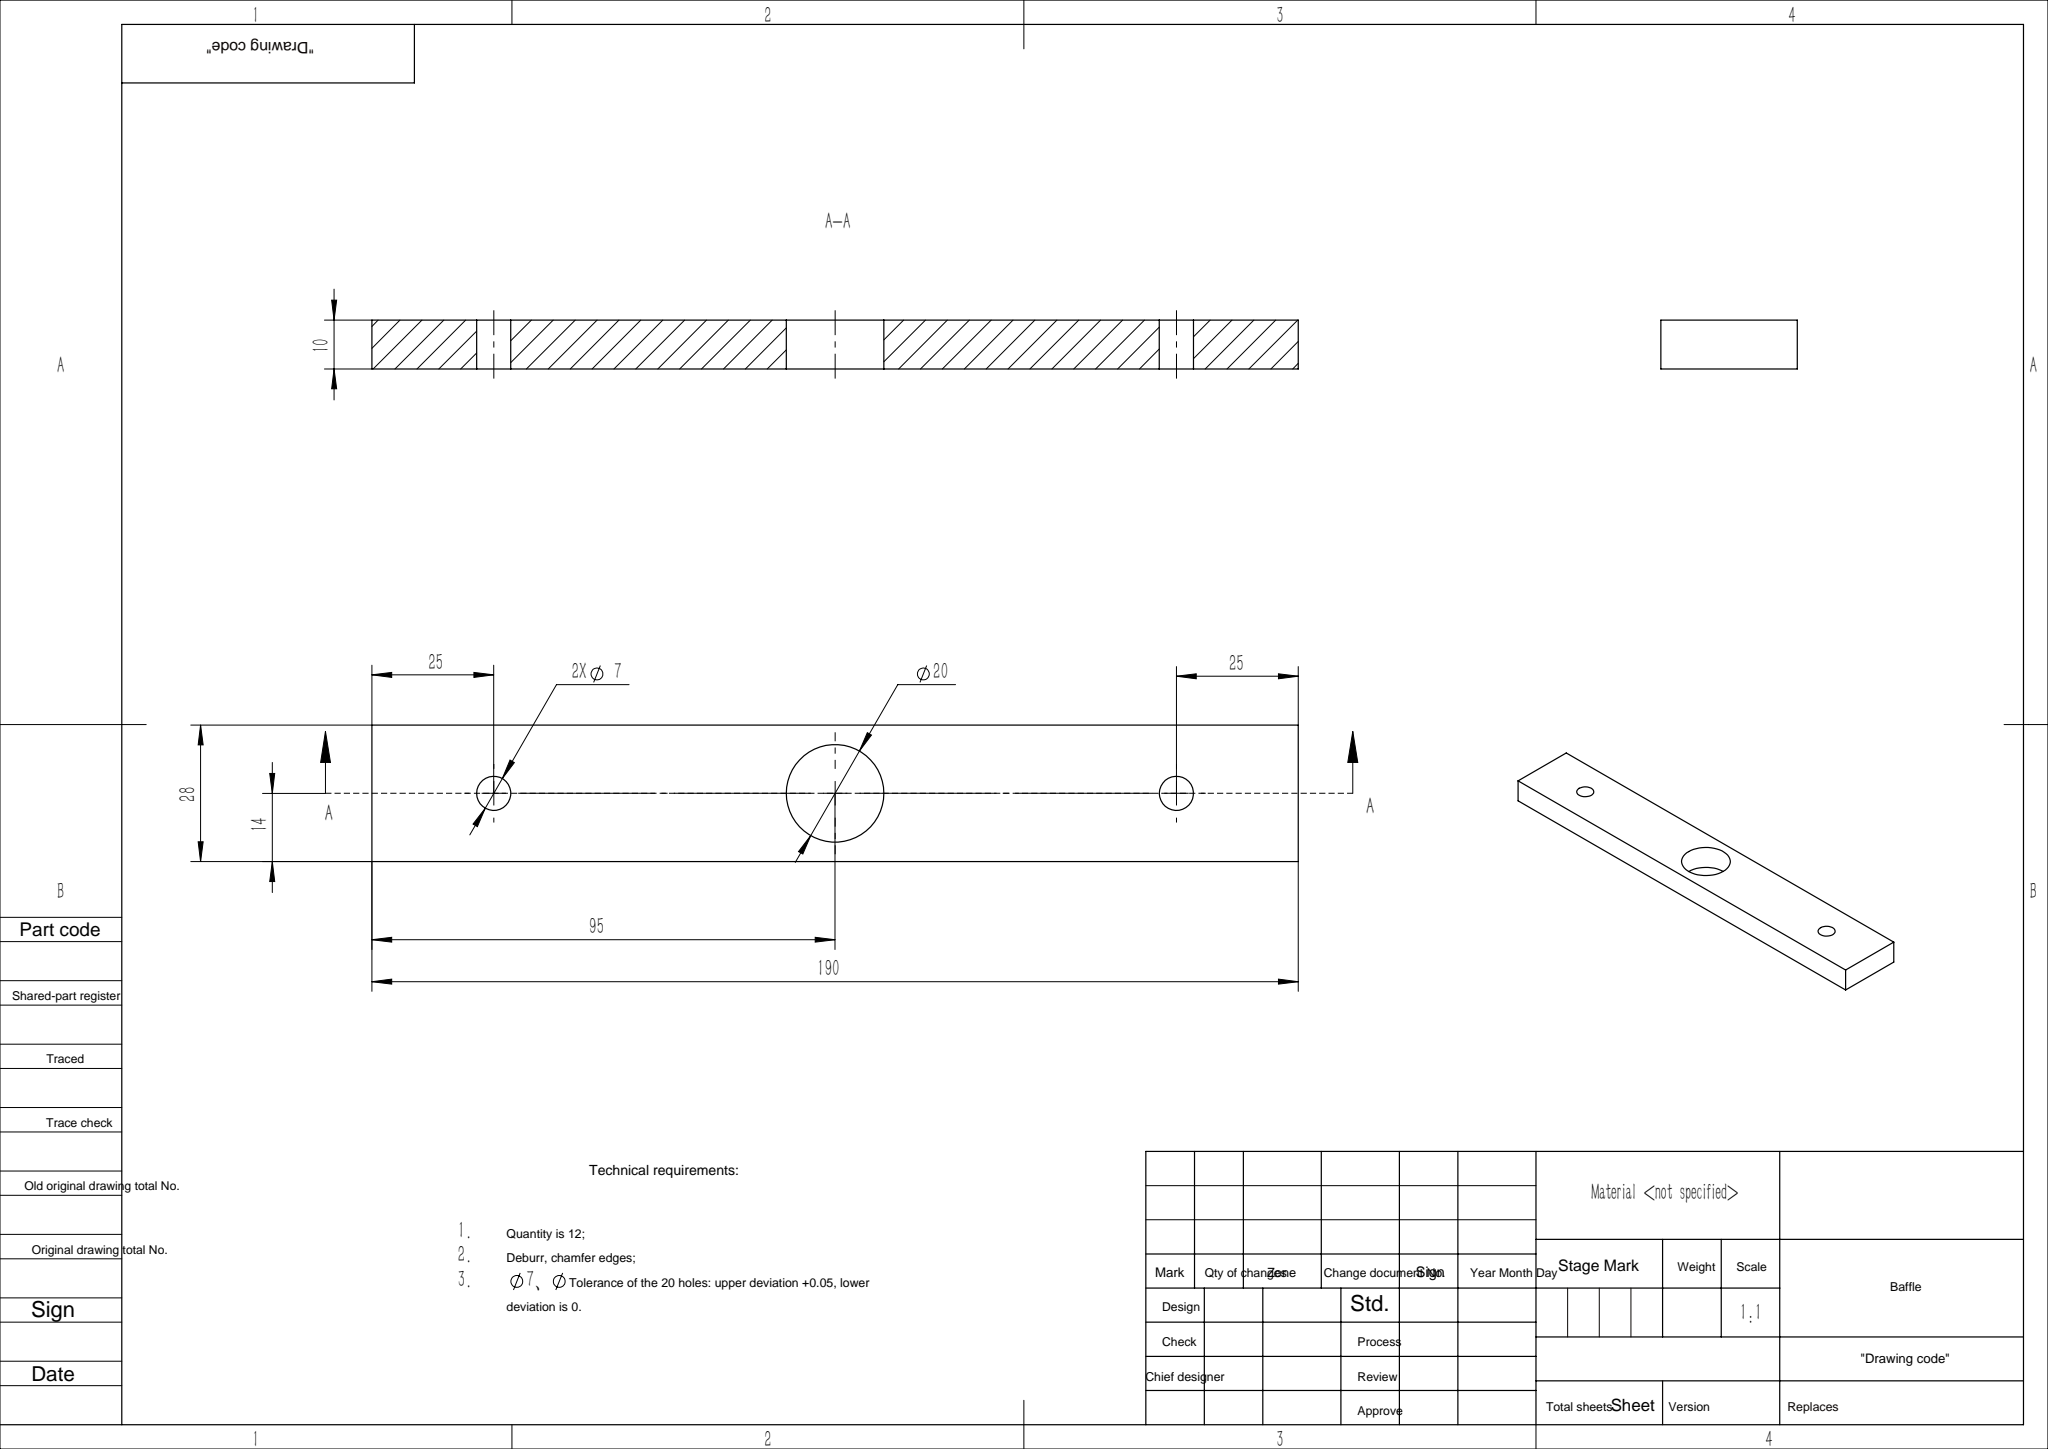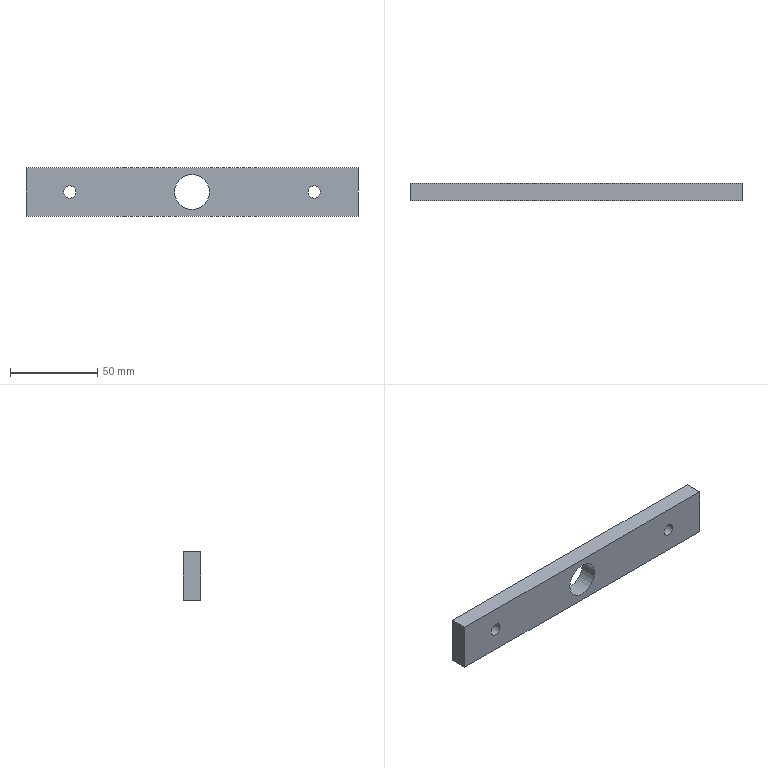Part | SolidWorks | features Cut 1, Extrusion 1 | 1 solid | 12 faces | box 190 x 10 x 28 mm | volume 49289 mm3 | cylinder 6 | plane 6 | commonest cylinder face diameters 7 x4 20 x2
STEP:
#1=CARTESIAN_POINT('',(612.086,1805.,-465.));
#2=VERTEX_POINT('',#1);
#3=CARTESIAN_POINT('',(592.086,1805.,-465.));
#4=VERTEX_POINT('',#3);
#5=CARTESIAN_POINT('',(602.086,1805.,-465.));
#6=DIRECTION('',(0.,1.,0.));
#7=DIRECTION('',(-1.,0.,0.));
#8=AXIS2_PLACEMENT_3D('',#5,#6,#7);
#9=CIRCLE('',#8,10.);
#10=EDGE_CURVE('',#2,#4,#9,.T.);
#11=ORIENTED_EDGE('',*,*,#10,.F.);
#12=CARTESIAN_POINT('',(612.086,1815.,-465.));
#13=VERTEX_POINT('',#12);
#14=CARTESIAN_POINT('',(612.086,1805.,-465.));
#15=DIRECTION('',(0.,1.,0.));
#16=VECTOR('',#15,1000.);
#17=LINE('',#14,#16);
#18=EDGE_CURVE('',#2,#13,#17,.T.);
#19=ORIENTED_EDGE('',*,*,#18,.T.);
#20=CARTESIAN_POINT('',(592.086,1815.,-465.));
#21=VERTEX_POINT('',#20);
#22=CARTESIAN_POINT('',(602.086,1815.,-465.));
#23=DIRECTION('',(0.,1.,0.));
#24=DIRECTION('',(-1.,0.,0.));
#25=AXIS2_PLACEMENT_3D('',#22,#23,#24);
#26=CIRCLE('',#25,10.);
#27=EDGE_CURVE('',#13,#21,#26,.T.);
#28=ORIENTED_EDGE('',*,*,#27,.T.);
#29=CARTESIAN_POINT('',(592.086,1805.,-465.));
#30=DIRECTION('',(0.,1.,0.));
#31=VECTOR('',#30,1000.);
#32=LINE('',#29,#31);
#33=EDGE_CURVE('',#4,#21,#32,.T.);
#34=ORIENTED_EDGE('',*,*,#33,.F.);
#35=EDGE_LOOP('',(#11,#19,#28,#34));
#36=FACE_OUTER_BOUND('',#35,.T.);
#37=CARTESIAN_POINT('',(602.086,1805.,-465.));
#38=DIRECTION('',(0.,1.,0.));
#39=DIRECTION('',(-1.,0.,0.));
#40=AXIS2_PLACEMENT_3D('',#37,#38,#39);
#41=CYLINDRICAL_SURFACE('',#40,10.);
#42=ADVANCED_FACE('',(#36),#41,.F.);
#43=CARTESIAN_POINT('',(675.586,1805.,-465.));
#44=VERTEX_POINT('',#43);
#45=CARTESIAN_POINT('',(668.586,1805.,-465.));
#46=VERTEX_POINT('',#45);
#47=CARTESIAN_POINT('',(672.086,1805.,-465.));
#48=DIRECTION('',(0.,1.,0.));
#49=DIRECTION('',(-1.,0.,0.));
#50=AXIS2_PLACEMENT_3D('',#47,#48,#49);
#51=CIRCLE('',#50,3.5);
#52=EDGE_CURVE('',#44,#46,#51,.T.);
#53=ORIENTED_EDGE('',*,*,#52,.F.);
#54=CARTESIAN_POINT('',(675.586,1815.,-465.));
#55=VERTEX_POINT('',#54);
#56=CARTESIAN_POINT('',(675.586,1805.,-465.));
#57=DIRECTION('',(0.,1.,0.));
#58=VECTOR('',#57,1000.);
#59=LINE('',#56,#58);
#60=EDGE_CURVE('',#44,#55,#59,.T.);
#61=ORIENTED_EDGE('',*,*,#60,.T.);
#62=CARTESIAN_POINT('',(668.586,1815.,-465.));
#63=VERTEX_POINT('',#62);
#64=CARTESIAN_POINT('',(672.086,1815.,-465.));
#65=DIRECTION('',(0.,1.,0.));
#66=DIRECTION('',(-1.,0.,0.));
#67=AXIS2_PLACEMENT_3D('',#64,#65,#66);
#68=CIRCLE('',#67,3.5);
#69=EDGE_CURVE('',#55,#63,#68,.T.);
#70=ORIENTED_EDGE('',*,*,#69,.T.);
#71=CARTESIAN_POINT('',(668.586,1805.,-465.));
#72=DIRECTION('',(0.,1.,0.));
#73=VECTOR('',#72,1000.);
#74=LINE('',#71,#73);
#75=EDGE_CURVE('',#46,#63,#74,.T.);
#76=ORIENTED_EDGE('',*,*,#75,.F.);
#77=EDGE_LOOP('',(#53,#61,#70,#76));
#78=FACE_OUTER_BOUND('',#77,.T.);
#79=CARTESIAN_POINT('',(672.086,1805.,-465.));
#80=DIRECTION('',(0.,1.,0.));
#81=DIRECTION('',(-1.,0.,0.));
#82=AXIS2_PLACEMENT_3D('',#79,#80,#81);
#83=CYLINDRICAL_SURFACE('',#82,3.5);
#84=ADVANCED_FACE('',(#78),#83,.F.);
#85=CARTESIAN_POINT('',(535.586,1805.,-465.));
#86=VERTEX_POINT('',#85);
#87=CARTESIAN_POINT('',(528.586,1805.,-465.));
#88=VERTEX_POINT('',#87);
#89=CARTESIAN_POINT('',(532.086,1805.,-465.));
#90=DIRECTION('',(0.,1.,0.));
#91=DIRECTION('',(-1.,0.,0.));
#92=AXIS2_PLACEMENT_3D('',#89,#90,#91);
#93=CIRCLE('',#92,3.5);
#94=EDGE_CURVE('',#86,#88,#93,.T.);
#95=ORIENTED_EDGE('',*,*,#94,.F.);
#96=CARTESIAN_POINT('',(535.586,1815.,-465.));
#97=VERTEX_POINT('',#96);
#98=CARTESIAN_POINT('',(535.586,1805.,-465.));
#99=DIRECTION('',(0.,1.,0.));
#100=VECTOR('',#99,1000.);
#101=LINE('',#98,#100);
#102=EDGE_CURVE('',#86,#97,#101,.T.);
#103=ORIENTED_EDGE('',*,*,#102,.T.);
#104=CARTESIAN_POINT('',(528.586,1815.,-465.));
#105=VERTEX_POINT('',#104);
#106=CARTESIAN_POINT('',(532.086,1815.,-465.));
#107=DIRECTION('',(0.,1.,0.));
#108=DIRECTION('',(-1.,0.,0.));
#109=AXIS2_PLACEMENT_3D('',#106,#107,#108);
#110=CIRCLE('',#109,3.5);
#111=EDGE_CURVE('',#97,#105,#110,.T.);
#112=ORIENTED_EDGE('',*,*,#111,.T.);
#113=CARTESIAN_POINT('',(528.586,1805.,-465.));
#114=DIRECTION('',(0.,1.,0.));
#115=VECTOR('',#114,1000.);
#116=LINE('',#113,#115);
#117=EDGE_CURVE('',#88,#105,#116,.T.);
#118=ORIENTED_EDGE('',*,*,#117,.F.);
#119=EDGE_LOOP('',(#95,#103,#112,#118));
#120=FACE_OUTER_BOUND('',#119,.T.);
#121=CARTESIAN_POINT('',(532.086,1805.,-465.));
#122=DIRECTION('',(0.,1.,0.));
#123=DIRECTION('',(-1.,0.,0.));
#124=AXIS2_PLACEMENT_3D('',#121,#122,#123);
#125=CYLINDRICAL_SURFACE('',#124,3.5);
#126=ADVANCED_FACE('',(#120),#125,.F.);
#127=CARTESIAN_POINT('',(507.086,1805.,-479.));
#128=VERTEX_POINT('',#127);
#129=CARTESIAN_POINT('',(507.086,1805.,-451.));
#130=VERTEX_POINT('',#129);
#131=CARTESIAN_POINT('',(507.086,1805.,-479.));
#132=DIRECTION('',(0.,0.,1.));
#133=VECTOR('',#132,1000.);
#134=LINE('',#131,#133);
#135=EDGE_CURVE('',#128,#130,#134,.T.);
#136=ORIENTED_EDGE('',*,*,#135,.T.);
#137=CARTESIAN_POINT('',(507.086,1815.,-451.));
#138=VERTEX_POINT('',#137);
#139=CARTESIAN_POINT('',(507.086,1815.,-451.));
#140=DIRECTION('',(0.,-1.,0.));
#141=VECTOR('',#140,1000.);
#142=LINE('',#139,#141);
#143=EDGE_CURVE('',#138,#130,#142,.T.);
#144=ORIENTED_EDGE('',*,*,#143,.F.);
#145=CARTESIAN_POINT('',(507.086,1815.,-479.));
#146=VERTEX_POINT('',#145);
#147=CARTESIAN_POINT('',(507.086,1815.,-479.));
#148=DIRECTION('',(0.,0.,1.));
#149=VECTOR('',#148,1000.);
#150=LINE('',#147,#149);
#151=EDGE_CURVE('',#146,#138,#150,.T.);
#152=ORIENTED_EDGE('',*,*,#151,.F.);
#153=CARTESIAN_POINT('',(507.086,1815.,-479.));
#154=DIRECTION('',(0.,-1.,0.));
#155=VECTOR('',#154,1000.);
#156=LINE('',#153,#155);
#157=EDGE_CURVE('',#146,#128,#156,.T.);
#158=ORIENTED_EDGE('',*,*,#157,.T.);
#159=EDGE_LOOP('',(#136,#144,#152,#158));
#160=FACE_OUTER_BOUND('',#159,.T.);
#161=CARTESIAN_POINT('',(507.086,1815.,-479.));
#162=DIRECTION('',(1.,0.,0.));
#163=DIRECTION('',(0.,1.,0.));
#164=AXIS2_PLACEMENT_3D('',#161,#162,#163);
#165=PLANE('',#164);
#166=ADVANCED_FACE('',(#160),#165,.F.);
#167=CARTESIAN_POINT('',(697.086,1805.,-451.));
#168=VERTEX_POINT('',#167);
#169=CARTESIAN_POINT('',(507.086,1805.,-451.));
#170=DIRECTION('',(1.,0.,0.));
#171=VECTOR('',#170,1000.);
#172=LINE('',#169,#171);
#173=EDGE_CURVE('',#130,#168,#172,.T.);
#174=ORIENTED_EDGE('',*,*,#173,.T.);
#175=CARTESIAN_POINT('',(697.086,1815.,-451.));
#176=VERTEX_POINT('',#175);
#177=CARTESIAN_POINT('',(697.086,1815.,-451.));
#178=DIRECTION('',(0.,-1.,0.));
#179=VECTOR('',#178,1000.);
#180=LINE('',#177,#179);
#181=EDGE_CURVE('',#176,#168,#180,.T.);
#182=ORIENTED_EDGE('',*,*,#181,.F.);
#183=CARTESIAN_POINT('',(507.086,1815.,-451.));
#184=DIRECTION('',(1.,0.,0.));
#185=VECTOR('',#184,1000.);
#186=LINE('',#183,#185);
#187=EDGE_CURVE('',#138,#176,#186,.T.);
#188=ORIENTED_EDGE('',*,*,#187,.F.);
#189=ORIENTED_EDGE('',*,*,#143,.T.);
#190=EDGE_LOOP('',(#174,#182,#188,#189));
#191=FACE_OUTER_BOUND('',#190,.T.);
#192=CARTESIAN_POINT('',(507.086,1815.,-451.));
#193=DIRECTION('',(0.,0.,-1.));
#194=DIRECTION('',(-1.,0.,0.));
#195=AXIS2_PLACEMENT_3D('',#192,#193,#194);
#196=PLANE('',#195);
#197=ADVANCED_FACE('',(#191),#196,.F.);
#198=CARTESIAN_POINT('',(697.086,1805.,-479.));
#199=VERTEX_POINT('',#198);
#200=CARTESIAN_POINT('',(697.086,1805.,-479.));
#201=DIRECTION('',(0.,0.,-1.));
#202=VECTOR('',#201,1000.);
#203=LINE('',#200,#202);
#204=EDGE_CURVE('',#168,#199,#203,.T.);
#205=ORIENTED_EDGE('',*,*,#204,.T.);
#206=CARTESIAN_POINT('',(697.086,1815.,-479.));
#207=VERTEX_POINT('',#206);
#208=CARTESIAN_POINT('',(697.086,1815.,-479.));
#209=DIRECTION('',(0.,-1.,0.));
#210=VECTOR('',#209,1000.);
#211=LINE('',#208,#210);
#212=EDGE_CURVE('',#207,#199,#211,.T.);
#213=ORIENTED_EDGE('',*,*,#212,.F.);
#214=CARTESIAN_POINT('',(697.086,1815.,-479.));
#215=DIRECTION('',(0.,0.,-1.));
#216=VECTOR('',#215,1000.);
#217=LINE('',#214,#216);
#218=EDGE_CURVE('',#176,#207,#217,.T.);
#219=ORIENTED_EDGE('',*,*,#218,.F.);
#220=ORIENTED_EDGE('',*,*,#181,.T.);
#221=EDGE_LOOP('',(#205,#213,#219,#220));
#222=FACE_OUTER_BOUND('',#221,.T.);
#223=CARTESIAN_POINT('',(697.086,1815.,-479.));
#224=DIRECTION('',(-1.,0.,0.));
#225=DIRECTION('',(0.,-1.,0.));
#226=AXIS2_PLACEMENT_3D('',#223,#224,#225);
#227=PLANE('',#226);
#228=ADVANCED_FACE('',(#222),#227,.F.);
#229=CARTESIAN_POINT('',(507.086,1805.,-479.));
#230=DIRECTION('',(-1.,0.,0.));
#231=VECTOR('',#230,1000.);
#232=LINE('',#229,#231);
#233=EDGE_CURVE('',#199,#128,#232,.T.);
#234=ORIENTED_EDGE('',*,*,#233,.T.);
#235=ORIENTED_EDGE('',*,*,#157,.F.);
#236=CARTESIAN_POINT('',(507.086,1815.,-479.));
#237=DIRECTION('',(-1.,0.,0.));
#238=VECTOR('',#237,1000.);
#239=LINE('',#236,#238);
#240=EDGE_CURVE('',#207,#146,#239,.T.);
#241=ORIENTED_EDGE('',*,*,#240,.F.);
#242=ORIENTED_EDGE('',*,*,#212,.T.);
#243=EDGE_LOOP('',(#234,#235,#241,#242));
#244=FACE_OUTER_BOUND('',#243,.T.);
#245=CARTESIAN_POINT('',(507.086,1815.,-479.));
#246=DIRECTION('',(0.,0.,1.));
#247=DIRECTION('',(1.,0.,0.));
#248=AXIS2_PLACEMENT_3D('',#245,#246,#247);
#249=PLANE('',#248);
#250=ADVANCED_FACE('',(#244),#249,.F.);
#251=CARTESIAN_POINT('',(602.086,1815.,-465.));
#252=DIRECTION('',(0.,1.,0.));
#253=DIRECTION('',(-1.,0.,0.));
#254=AXIS2_PLACEMENT_3D('',#251,#252,#253);
#255=CIRCLE('',#254,10.);
#256=EDGE_CURVE('',#21,#13,#255,.T.);
#257=ORIENTED_EDGE('',*,*,#256,.F.);
#258=ORIENTED_EDGE('',*,*,#27,.F.);
#259=EDGE_LOOP('',(#257,#258));
#260=FACE_BOUND('',#259,.T.);
#261=CARTESIAN_POINT('',(672.086,1815.,-465.));
#262=DIRECTION('',(0.,1.,0.));
#263=DIRECTION('',(-1.,0.,0.));
#264=AXIS2_PLACEMENT_3D('',#261,#262,#263);
#265=CIRCLE('',#264,3.5);
#266=EDGE_CURVE('',#63,#55,#265,.T.);
#267=ORIENTED_EDGE('',*,*,#266,.F.);
#268=ORIENTED_EDGE('',*,*,#69,.F.);
#269=EDGE_LOOP('',(#267,#268));
#270=FACE_BOUND('',#269,.T.);
#271=CARTESIAN_POINT('',(532.086,1815.,-465.));
#272=DIRECTION('',(0.,1.,0.));
#273=DIRECTION('',(-1.,0.,0.));
#274=AXIS2_PLACEMENT_3D('',#271,#272,#273);
#275=CIRCLE('',#274,3.5);
#276=EDGE_CURVE('',#105,#97,#275,.T.);
#277=ORIENTED_EDGE('',*,*,#276,.F.);
#278=ORIENTED_EDGE('',*,*,#111,.F.);
#279=EDGE_LOOP('',(#277,#278));
#280=FACE_BOUND('',#279,.T.);
#281=ORIENTED_EDGE('',*,*,#151,.T.);
#282=ORIENTED_EDGE('',*,*,#187,.T.);
#283=ORIENTED_EDGE('',*,*,#218,.T.);
#284=ORIENTED_EDGE('',*,*,#240,.T.);
#285=EDGE_LOOP('',(#281,#282,#283,#284));
#286=FACE_OUTER_BOUND('',#285,.T.);
#287=CARTESIAN_POINT('',(0.,1815.,0.));
#288=DIRECTION('',(0.,1.,0.));
#289=DIRECTION('',(-1.,0.,0.));
#290=AXIS2_PLACEMENT_3D('',#287,#288,#289);
#291=PLANE('',#290);
#292=ADVANCED_FACE('',(#260,#270,#280,#286),#291,.T.);
#293=CARTESIAN_POINT('',(602.086,1805.,-465.));
#294=DIRECTION('',(0.,1.,0.));
#295=DIRECTION('',(-1.,0.,0.));
#296=AXIS2_PLACEMENT_3D('',#293,#294,#295);
#297=CIRCLE('',#296,10.);
#298=EDGE_CURVE('',#4,#2,#297,.T.);
#299=ORIENTED_EDGE('',*,*,#298,.T.);
#300=ORIENTED_EDGE('',*,*,#10,.T.);
#301=EDGE_LOOP('',(#299,#300));
#302=FACE_BOUND('',#301,.T.);
#303=CARTESIAN_POINT('',(672.086,1805.,-465.));
#304=DIRECTION('',(0.,1.,0.));
#305=DIRECTION('',(-1.,0.,0.));
#306=AXIS2_PLACEMENT_3D('',#303,#304,#305);
#307=CIRCLE('',#306,3.5);
#308=EDGE_CURVE('',#46,#44,#307,.T.);
#309=ORIENTED_EDGE('',*,*,#308,.T.);
#310=ORIENTED_EDGE('',*,*,#52,.T.);
#311=EDGE_LOOP('',(#309,#310));
#312=FACE_BOUND('',#311,.T.);
#313=CARTESIAN_POINT('',(532.086,1805.,-465.));
#314=DIRECTION('',(0.,1.,0.));
#315=DIRECTION('',(-1.,0.,0.));
#316=AXIS2_PLACEMENT_3D('',#313,#314,#315);
#317=CIRCLE('',#316,3.5);
#318=EDGE_CURVE('',#88,#86,#317,.T.);
#319=ORIENTED_EDGE('',*,*,#318,.T.);
#320=ORIENTED_EDGE('',*,*,#94,.T.);
#321=EDGE_LOOP('',(#319,#320));
#322=FACE_BOUND('',#321,.T.);
#323=ORIENTED_EDGE('',*,*,#135,.F.);
#324=ORIENTED_EDGE('',*,*,#233,.F.);
#325=ORIENTED_EDGE('',*,*,#204,.F.);
#326=ORIENTED_EDGE('',*,*,#173,.F.);
#327=EDGE_LOOP('',(#323,#324,#325,#326));
#328=FACE_OUTER_BOUND('',#327,.T.);
#329=CARTESIAN_POINT('',(0.,1805.,0.));
#330=DIRECTION('',(0.,1.,0.));
#331=DIRECTION('',(-1.,0.,0.));
#332=AXIS2_PLACEMENT_3D('',#329,#330,#331);
#333=PLANE('',#332);
#334=ADVANCED_FACE('',(#302,#312,#322,#328),#333,.F.);
#335=ORIENTED_EDGE('',*,*,#102,.F.);
#336=ORIENTED_EDGE('',*,*,#318,.F.);
#337=ORIENTED_EDGE('',*,*,#117,.T.);
#338=ORIENTED_EDGE('',*,*,#276,.T.);
#339=EDGE_LOOP('',(#335,#336,#337,#338));
#340=FACE_OUTER_BOUND('',#339,.T.);
#341=CARTESIAN_POINT('',(532.086,1805.,-465.));
#342=DIRECTION('',(0.,1.,0.));
#343=DIRECTION('',(-1.,0.,0.));
#344=AXIS2_PLACEMENT_3D('',#341,#342,#343);
#345=CYLINDRICAL_SURFACE('',#344,3.5);
#346=ADVANCED_FACE('',(#340),#345,.F.);
#347=ORIENTED_EDGE('',*,*,#60,.F.);
#348=ORIENTED_EDGE('',*,*,#308,.F.);
#349=ORIENTED_EDGE('',*,*,#75,.T.);
#350=ORIENTED_EDGE('',*,*,#266,.T.);
#351=EDGE_LOOP('',(#347,#348,#349,#350));
#352=FACE_OUTER_BOUND('',#351,.T.);
#353=CARTESIAN_POINT('',(672.086,1805.,-465.));
#354=DIRECTION('',(0.,1.,0.));
#355=DIRECTION('',(-1.,0.,0.));
#356=AXIS2_PLACEMENT_3D('',#353,#354,#355);
#357=CYLINDRICAL_SURFACE('',#356,3.5);
#358=ADVANCED_FACE('',(#352),#357,.F.);
#359=ORIENTED_EDGE('',*,*,#18,.F.);
#360=ORIENTED_EDGE('',*,*,#298,.F.);
#361=ORIENTED_EDGE('',*,*,#33,.T.);
#362=ORIENTED_EDGE('',*,*,#256,.T.);
#363=EDGE_LOOP('',(#359,#360,#361,#362));
#364=FACE_OUTER_BOUND('',#363,.T.);
#365=CARTESIAN_POINT('',(602.086,1805.,-465.));
#366=DIRECTION('',(0.,1.,0.));
#367=DIRECTION('',(-1.,0.,0.));
#368=AXIS2_PLACEMENT_3D('',#365,#366,#367);
#369=CYLINDRICAL_SURFACE('',#368,10.);
#370=ADVANCED_FACE('',(#364),#369,.F.);
#371=CLOSED_SHELL('',(#42,#84,#126,#166,#197,#228,#250,#292,#334,#346,#358,#370));
#372=MANIFOLD_SOLID_BREP('',#371);
#373=CARTESIAN_POINT('',(0.,0.,0.));
#374=DIRECTION('',(0.,0.,1.));
#375=DIRECTION('',(1.,0.,0.));
#376=AXIS2_PLACEMENT_3D('',#373,#374,#375);
#377=(LENGTH_UNIT()NAMED_UNIT(*)SI_UNIT(.MILLI.,.METRE.));
#378=UNCERTAINTY_MEASURE_WITH_UNIT(LENGTH_MEASURE(0.00001),#377,'','');
#379=(NAMED_UNIT(*)PLANE_ANGLE_UNIT()SI_UNIT($,.RADIAN.));
#380=(NAMED_UNIT(*)SI_UNIT($,.STERADIAN.)SOLID_ANGLE_UNIT());
#381=(GEOMETRIC_REPRESENTATION_CONTEXT(3)GLOBAL_UNCERTAINTY_ASSIGNED_CONTEXT((#378))GLOBAL_UNIT_ASSIGNED_CONTEXT((#377,#379,#380))REPRESENTATION_CONTEXT('',''));
#382=ADVANCED_BREP_SHAPE_REPRESENTATION('',(#372,#376),#381);